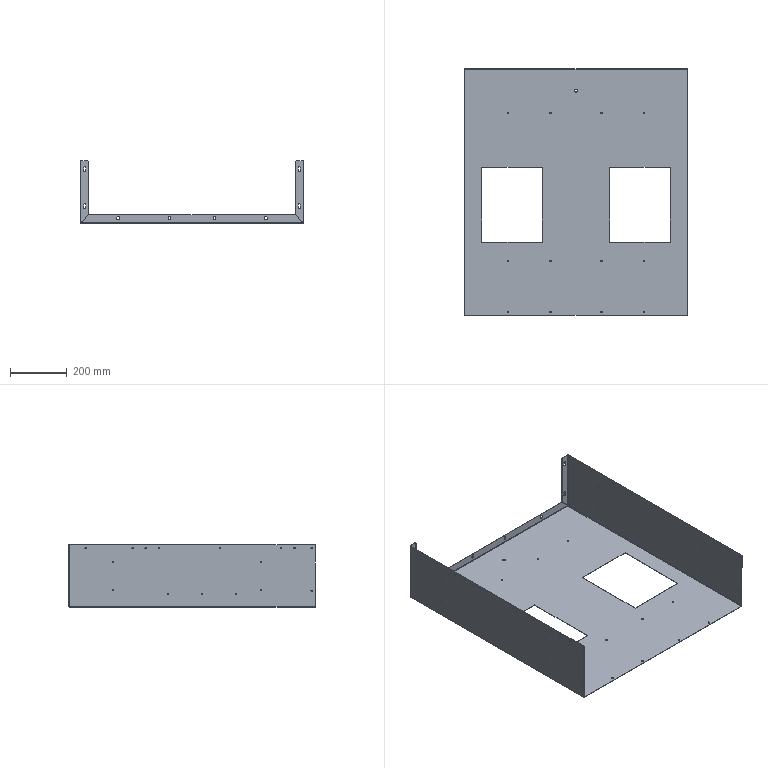Part | SolidWorks | features ICE 6, HoleWzd 5, EdgeFlange 4, LPattern 2, Fillet 1, FlatPattern 1, SMBaseFlange 1, SheetMetal 1 | 1 solid | 182 faces | box 787 x 866 x 220 mm | volume 1173690 mm3 | cylinder 122 | plane 56 | spline 4 | commonest cylinder face diameters 5 x72 8 x20 4 x12 2 x5 4.4 x5 6 x4